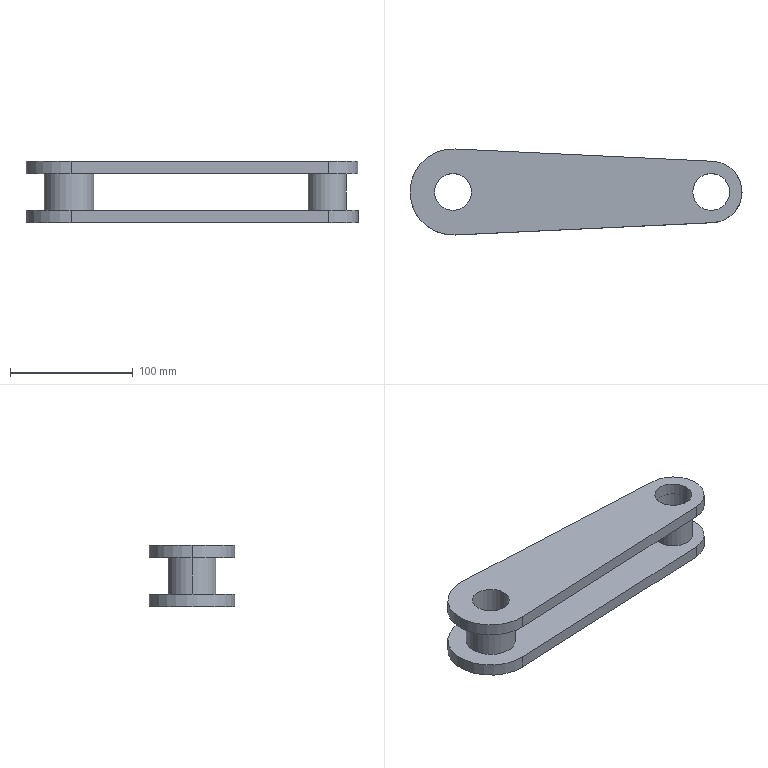Part | SolidWorks | features ICE 4, Extrusion 1 | 2 solids | 28 faces | box 270 x 70 x 50 mm | volume 300062 mm3 | cylinder 18 | plane 10 | commonest cylinder face diameters 30 x8 50 x3 70 x3 31 x2 40 x2
STEP:
#1=CARTESIAN_POINT('',(225.,0.,-30.));
#2=VERTEX_POINT('',#1);
#3=CARTESIAN_POINT('',(195.,0.,-30.));
#4=VERTEX_POINT('',#3);
#5=CARTESIAN_POINT('',(210.,0.,-30.));
#6=DIRECTION('',(0.,0.,-1.));
#7=DIRECTION('',(-1.,0.,0.));
#8=AXIS2_PLACEMENT_3D('',#5,#6,#7);
#9=CIRCLE('',#8,15.);
#10=EDGE_CURVE('',#2,#4,#9,.T.);
#11=ORIENTED_EDGE('',*,*,#10,.T.);
#12=CARTESIAN_POINT('',(195.,0.,10.));
#13=VERTEX_POINT('',#12);
#14=CARTESIAN_POINT('',(195.,0.,-30.));
#15=DIRECTION('',(0.,0.,1.));
#16=VECTOR('',#15,1000.);
#17=LINE('',#14,#16);
#18=EDGE_CURVE('',#4,#13,#17,.T.);
#19=ORIENTED_EDGE('',*,*,#18,.T.);
#20=CARTESIAN_POINT('',(225.,0.,10.));
#21=VERTEX_POINT('',#20);
#22=CARTESIAN_POINT('',(210.,0.,10.));
#23=DIRECTION('',(0.,0.,1.));
#24=DIRECTION('',(1.,0.,0.));
#25=AXIS2_PLACEMENT_3D('',#22,#23,#24);
#26=CIRCLE('',#25,15.);
#27=EDGE_CURVE('',#13,#21,#26,.T.);
#28=ORIENTED_EDGE('',*,*,#27,.T.);
#29=CARTESIAN_POINT('',(225.,0.,-30.));
#30=DIRECTION('',(0.,0.,1.));
#31=VECTOR('',#30,1000.);
#32=LINE('',#29,#31);
#33=EDGE_CURVE('',#2,#21,#32,.T.);
#34=ORIENTED_EDGE('',*,*,#33,.F.);
#35=EDGE_LOOP('',(#11,#19,#28,#34));
#36=FACE_OUTER_BOUND('',#35,.T.);
#37=CARTESIAN_POINT('',(210.,0.,-30.));
#38=DIRECTION('',(0.,0.,1.));
#39=DIRECTION('',(1.,0.,0.));
#40=AXIS2_PLACEMENT_3D('',#37,#38,#39);
#41=CYLINDRICAL_SURFACE('',#40,15.);
#42=ADVANCED_FACE('',(#36),#41,.F.);
#43=CARTESIAN_POINT('',(194.5,0.,-30.));
#44=VERTEX_POINT('',#43);
#45=CARTESIAN_POINT('',(225.5,0.,-30.));
#46=VERTEX_POINT('',#45);
#47=CARTESIAN_POINT('',(210.,0.,-30.));
#48=DIRECTION('',(0.,0.,-1.));
#49=DIRECTION('',(-1.,0.,0.));
#50=AXIS2_PLACEMENT_3D('',#47,#48,#49);
#51=CIRCLE('',#50,15.5);
#52=EDGE_CURVE('',#44,#46,#51,.T.);
#53=ORIENTED_EDGE('',*,*,#52,.F.);
#54=CARTESIAN_POINT('',(194.5,0.,0.));
#55=VERTEX_POINT('',#54);
#56=CARTESIAN_POINT('',(194.5,0.,-30.));
#57=DIRECTION('',(0.,0.,1.));
#58=VECTOR('',#57,1000.);
#59=LINE('',#56,#58);
#60=EDGE_CURVE('',#44,#55,#59,.T.);
#61=ORIENTED_EDGE('',*,*,#60,.T.);
#62=CARTESIAN_POINT('',(225.5,0.,0.));
#63=VERTEX_POINT('',#62);
#64=CARTESIAN_POINT('',(210.,0.,0.));
#65=DIRECTION('',(0.,0.,-1.));
#66=DIRECTION('',(1.,0.,0.));
#67=AXIS2_PLACEMENT_3D('',#64,#65,#66);
#68=CIRCLE('',#67,15.5);
#69=EDGE_CURVE('',#55,#63,#68,.T.);
#70=ORIENTED_EDGE('',*,*,#69,.T.);
#71=CARTESIAN_POINT('',(225.5,0.,-30.));
#72=DIRECTION('',(0.,0.,1.));
#73=VECTOR('',#72,1000.);
#74=LINE('',#71,#73);
#75=EDGE_CURVE('',#46,#63,#74,.T.);
#76=ORIENTED_EDGE('',*,*,#75,.F.);
#77=EDGE_LOOP('',(#53,#61,#70,#76));
#78=FACE_OUTER_BOUND('',#77,.T.);
#79=CARTESIAN_POINT('',(210.,0.,-30.));
#80=DIRECTION('',(0.,0.,1.));
#81=DIRECTION('',(1.,0.,0.));
#82=AXIS2_PLACEMENT_3D('',#79,#80,#81);
#83=CYLINDRICAL_SURFACE('',#82,15.5);
#84=ADVANCED_FACE('',(#78),#83,.T.);
#85=CARTESIAN_POINT('',(15.,0.,-30.));
#86=VERTEX_POINT('',#85);
#87=CARTESIAN_POINT('',(-15.,0.,-30.));
#88=VERTEX_POINT('',#87);
#89=CARTESIAN_POINT('',(0.,0.,-30.));
#90=DIRECTION('',(0.,0.,-1.));
#91=DIRECTION('',(-1.,0.,0.));
#92=AXIS2_PLACEMENT_3D('',#89,#90,#91);
#93=CIRCLE('',#92,15.);
#94=EDGE_CURVE('',#86,#88,#93,.T.);
#95=ORIENTED_EDGE('',*,*,#94,.T.);
#96=CARTESIAN_POINT('',(-15.,0.,10.));
#97=VERTEX_POINT('',#96);
#98=CARTESIAN_POINT('',(-15.,0.,-30.));
#99=DIRECTION('',(0.,0.,1.));
#100=VECTOR('',#99,1000.);
#101=LINE('',#98,#100);
#102=EDGE_CURVE('',#88,#97,#101,.T.);
#103=ORIENTED_EDGE('',*,*,#102,.T.);
#104=CARTESIAN_POINT('',(15.,0.,10.));
#105=VERTEX_POINT('',#104);
#106=CARTESIAN_POINT('',(0.,0.,10.));
#107=DIRECTION('',(0.,0.,1.));
#108=DIRECTION('',(1.,0.,0.));
#109=AXIS2_PLACEMENT_3D('',#106,#107,#108);
#110=CIRCLE('',#109,15.);
#111=EDGE_CURVE('',#97,#105,#110,.T.);
#112=ORIENTED_EDGE('',*,*,#111,.T.);
#113=CARTESIAN_POINT('',(15.,0.,-30.));
#114=DIRECTION('',(0.,0.,1.));
#115=VECTOR('',#114,1000.);
#116=LINE('',#113,#115);
#117=EDGE_CURVE('',#86,#105,#116,.T.);
#118=ORIENTED_EDGE('',*,*,#117,.F.);
#119=EDGE_LOOP('',(#95,#103,#112,#118));
#120=FACE_OUTER_BOUND('',#119,.T.);
#121=CARTESIAN_POINT('',(0.,0.,-30.));
#122=DIRECTION('',(0.,0.,1.));
#123=DIRECTION('',(1.,0.,0.));
#124=AXIS2_PLACEMENT_3D('',#121,#122,#123);
#125=CYLINDRICAL_SURFACE('',#124,15.);
#126=ADVANCED_FACE('',(#120),#125,.F.);
#127=CARTESIAN_POINT('',(-20.,0.,-30.));
#128=VERTEX_POINT('',#127);
#129=CARTESIAN_POINT('',(20.,0.,-30.));
#130=VERTEX_POINT('',#129);
#131=CARTESIAN_POINT('',(0.,0.,-30.));
#132=DIRECTION('',(0.,0.,-1.));
#133=DIRECTION('',(-1.,0.,0.));
#134=AXIS2_PLACEMENT_3D('',#131,#132,#133);
#135=CIRCLE('',#134,20.);
#136=EDGE_CURVE('',#128,#130,#135,.T.);
#137=ORIENTED_EDGE('',*,*,#136,.F.);
#138=CARTESIAN_POINT('',(-20.,0.,0.));
#139=VERTEX_POINT('',#138);
#140=CARTESIAN_POINT('',(-20.,0.,-30.));
#141=DIRECTION('',(0.,0.,1.));
#142=VECTOR('',#141,1000.);
#143=LINE('',#140,#142);
#144=EDGE_CURVE('',#128,#139,#143,.T.);
#145=ORIENTED_EDGE('',*,*,#144,.T.);
#146=CARTESIAN_POINT('',(20.,0.,0.));
#147=VERTEX_POINT('',#146);
#148=CARTESIAN_POINT('',(0.,0.,0.));
#149=DIRECTION('',(0.,0.,-1.));
#150=DIRECTION('',(1.,0.,0.));
#151=AXIS2_PLACEMENT_3D('',#148,#149,#150);
#152=CIRCLE('',#151,20.);
#153=EDGE_CURVE('',#139,#147,#152,.T.);
#154=ORIENTED_EDGE('',*,*,#153,.T.);
#155=CARTESIAN_POINT('',(20.,0.,-30.));
#156=DIRECTION('',(0.,0.,1.));
#157=VECTOR('',#156,1000.);
#158=LINE('',#155,#157);
#159=EDGE_CURVE('',#130,#147,#158,.T.);
#160=ORIENTED_EDGE('',*,*,#159,.F.);
#161=EDGE_LOOP('',(#137,#145,#154,#160));
#162=FACE_OUTER_BOUND('',#161,.T.);
#163=CARTESIAN_POINT('',(0.,0.,-30.));
#164=DIRECTION('',(0.,0.,1.));
#165=DIRECTION('',(1.,0.,0.));
#166=AXIS2_PLACEMENT_3D('',#163,#164,#165);
#167=CYLINDRICAL_SURFACE('',#166,20.);
#168=ADVANCED_FACE('',(#162),#167,.T.);
#169=CARTESIAN_POINT('',(-35.,0.,10.));
#170=VERTEX_POINT('',#169);
#171=CARTESIAN_POINT('',(1.667,-34.96,10.));
#172=VERTEX_POINT('',#171);
#173=CARTESIAN_POINT('',(0.,0.,10.));
#174=DIRECTION('',(0.,0.,1.));
#175=DIRECTION('',(1.,0.,0.));
#176=AXIS2_PLACEMENT_3D('',#173,#174,#175);
#177=CIRCLE('',#176,35.);
#178=EDGE_CURVE('',#170,#172,#177,.T.);
#179=ORIENTED_EDGE('',*,*,#178,.F.);
#180=CARTESIAN_POINT('',(-35.,0.,0.));
#181=VERTEX_POINT('',#180);
#182=CARTESIAN_POINT('',(-35.,0.,10.));
#183=DIRECTION('',(0.,0.,-1.));
#184=VECTOR('',#183,1000.);
#185=LINE('',#182,#184);
#186=EDGE_CURVE('',#170,#181,#185,.T.);
#187=ORIENTED_EDGE('',*,*,#186,.T.);
#188=CARTESIAN_POINT('',(1.667,-34.96,0.));
#189=VERTEX_POINT('',#188);
#190=CARTESIAN_POINT('',(0.,0.,0.));
#191=DIRECTION('',(0.,0.,1.));
#192=DIRECTION('',(1.,0.,0.));
#193=AXIS2_PLACEMENT_3D('',#190,#191,#192);
#194=CIRCLE('',#193,35.);
#195=EDGE_CURVE('',#181,#189,#194,.T.);
#196=ORIENTED_EDGE('',*,*,#195,.T.);
#197=CARTESIAN_POINT('',(1.667,-34.96,10.));
#198=DIRECTION('',(0.,0.,-1.));
#199=VECTOR('',#198,1000.);
#200=LINE('',#197,#199);
#201=EDGE_CURVE('',#172,#189,#200,.T.);
#202=ORIENTED_EDGE('',*,*,#201,.F.);
#203=EDGE_LOOP('',(#179,#187,#196,#202));
#204=FACE_OUTER_BOUND('',#203,.T.);
#205=CARTESIAN_POINT('',(0.,0.,10.));
#206=DIRECTION('',(0.,0.,-1.));
#207=DIRECTION('',(-1.,0.,0.));
#208=AXIS2_PLACEMENT_3D('',#205,#206,#207);
#209=CYLINDRICAL_SURFACE('',#208,35.);
#210=ADVANCED_FACE('',(#204),#209,.T.);
#211=ORIENTED_EDGE('',*,*,#186,.F.);
#212=CARTESIAN_POINT('',(1.667,34.96,10.));
#213=VERTEX_POINT('',#212);
#214=CARTESIAN_POINT('',(0.,0.,10.));
#215=DIRECTION('',(0.,0.,1.));
#216=DIRECTION('',(1.,0.,0.));
#217=AXIS2_PLACEMENT_3D('',#214,#215,#216);
#218=CIRCLE('',#217,35.);
#219=EDGE_CURVE('',#213,#170,#218,.T.);
#220=ORIENTED_EDGE('',*,*,#219,.F.);
#221=CARTESIAN_POINT('',(1.667,34.96,0.));
#222=VERTEX_POINT('',#221);
#223=CARTESIAN_POINT('',(1.667,34.96,10.));
#224=DIRECTION('',(0.,0.,-1.));
#225=VECTOR('',#224,1000.);
#226=LINE('',#223,#225);
#227=EDGE_CURVE('',#213,#222,#226,.T.);
#228=ORIENTED_EDGE('',*,*,#227,.T.);
#229=CARTESIAN_POINT('',(0.,0.,0.));
#230=DIRECTION('',(0.,0.,1.));
#231=DIRECTION('',(1.,0.,0.));
#232=AXIS2_PLACEMENT_3D('',#229,#230,#231);
#233=CIRCLE('',#232,35.);
#234=EDGE_CURVE('',#222,#181,#233,.T.);
#235=ORIENTED_EDGE('',*,*,#234,.T.);
#236=EDGE_LOOP('',(#211,#220,#228,#235));
#237=FACE_OUTER_BOUND('',#236,.T.);
#238=CARTESIAN_POINT('',(0.,0.,10.));
#239=DIRECTION('',(0.,0.,-1.));
#240=DIRECTION('',(-1.,0.,0.));
#241=AXIS2_PLACEMENT_3D('',#238,#239,#240);
#242=CYLINDRICAL_SURFACE('',#241,35.);
#243=ADVANCED_FACE('',(#237),#242,.T.);
#244=CARTESIAN_POINT('',(211.19,-24.972,0.));
#245=VERTEX_POINT('',#244);
#246=CARTESIAN_POINT('',(1.667,-34.96,0.));
#247=DIRECTION('',(0.9989,0.04762,0.));
#248=VECTOR('',#247,1000.);
#249=LINE('',#246,#248);
#250=EDGE_CURVE('',#189,#245,#249,.T.);
#251=ORIENTED_EDGE('',*,*,#250,.T.);
#252=CARTESIAN_POINT('',(211.19,-24.972,10.));
#253=VERTEX_POINT('',#252);
#254=CARTESIAN_POINT('',(211.19,-24.972,10.));
#255=DIRECTION('',(0.,0.,-1.));
#256=VECTOR('',#255,1000.);
#257=LINE('',#254,#256);
#258=EDGE_CURVE('',#253,#245,#257,.T.);
#259=ORIENTED_EDGE('',*,*,#258,.F.);
#260=CARTESIAN_POINT('',(1.667,-34.96,10.));
#261=DIRECTION('',(0.9989,0.04762,0.));
#262=VECTOR('',#261,1000.);
#263=LINE('',#260,#262);
#264=EDGE_CURVE('',#172,#253,#263,.T.);
#265=ORIENTED_EDGE('',*,*,#264,.F.);
#266=ORIENTED_EDGE('',*,*,#201,.T.);
#267=EDGE_LOOP('',(#251,#259,#265,#266));
#268=FACE_OUTER_BOUND('',#267,.T.);
#269=CARTESIAN_POINT('',(1.667,-34.96,10.));
#270=DIRECTION('',(-0.04762,0.9989,0.));
#271=DIRECTION('',(-0.9989,-0.04762,0.));
#272=AXIS2_PLACEMENT_3D('',#269,#270,#271);
#273=PLANE('',#272);
#274=ADVANCED_FACE('',(#268),#273,.F.);
#275=CARTESIAN_POINT('',(211.19,24.972,0.));
#276=VERTEX_POINT('',#275);
#277=CARTESIAN_POINT('',(210.,0.,0.));
#278=DIRECTION('',(0.,0.,1.));
#279=DIRECTION('',(1.,0.,0.));
#280=AXIS2_PLACEMENT_3D('',#277,#278,#279);
#281=CIRCLE('',#280,25.);
#282=EDGE_CURVE('',#245,#276,#281,.T.);
#283=ORIENTED_EDGE('',*,*,#282,.T.);
#284=CARTESIAN_POINT('',(211.19,24.972,10.));
#285=VERTEX_POINT('',#284);
#286=CARTESIAN_POINT('',(211.19,24.972,10.));
#287=DIRECTION('',(0.,0.,-1.));
#288=VECTOR('',#287,1000.);
#289=LINE('',#286,#288);
#290=EDGE_CURVE('',#285,#276,#289,.T.);
#291=ORIENTED_EDGE('',*,*,#290,.F.);
#292=CARTESIAN_POINT('',(210.,0.,10.));
#293=DIRECTION('',(0.,0.,1.));
#294=DIRECTION('',(1.,0.,0.));
#295=AXIS2_PLACEMENT_3D('',#292,#293,#294);
#296=CIRCLE('',#295,25.);
#297=EDGE_CURVE('',#253,#285,#296,.T.);
#298=ORIENTED_EDGE('',*,*,#297,.F.);
#299=ORIENTED_EDGE('',*,*,#258,.T.);
#300=EDGE_LOOP('',(#283,#291,#298,#299));
#301=FACE_OUTER_BOUND('',#300,.T.);
#302=CARTESIAN_POINT('',(210.,0.,10.));
#303=DIRECTION('',(0.,0.,-1.));
#304=DIRECTION('',(-1.,0.,0.));
#305=AXIS2_PLACEMENT_3D('',#302,#303,#304);
#306=CYLINDRICAL_SURFACE('',#305,25.);
#307=ADVANCED_FACE('',(#301),#306,.T.);
#308=CARTESIAN_POINT('',(1.667,34.96,0.));
#309=DIRECTION('',(-0.9989,0.04762,0.));
#310=VECTOR('',#309,1000.);
#311=LINE('',#308,#310);
#312=EDGE_CURVE('',#276,#222,#311,.T.);
#313=ORIENTED_EDGE('',*,*,#312,.T.);
#314=ORIENTED_EDGE('',*,*,#227,.F.);
#315=CARTESIAN_POINT('',(1.667,34.96,10.));
#316=DIRECTION('',(-0.9989,0.04762,0.));
#317=VECTOR('',#316,1000.);
#318=LINE('',#315,#317);
#319=EDGE_CURVE('',#285,#213,#318,.T.);
#320=ORIENTED_EDGE('',*,*,#319,.F.);
#321=ORIENTED_EDGE('',*,*,#290,.T.);
#322=EDGE_LOOP('',(#313,#314,#320,#321));
#323=FACE_OUTER_BOUND('',#322,.T.);
#324=CARTESIAN_POINT('',(1.667,34.96,10.));
#325=DIRECTION('',(-0.04762,-0.9989,0.));
#326=DIRECTION('',(0.9989,-0.04762,0.));
#327=AXIS2_PLACEMENT_3D('',#324,#325,#326);
#328=PLANE('',#327);
#329=ADVANCED_FACE('',(#323),#328,.F.);
#330=CARTESIAN_POINT('',(210.,0.,10.));
#331=DIRECTION('',(0.,0.,1.));
#332=DIRECTION('',(1.,0.,0.));
#333=AXIS2_PLACEMENT_3D('',#330,#331,#332);
#334=CIRCLE('',#333,15.);
#335=EDGE_CURVE('',#21,#13,#334,.T.);
#336=ORIENTED_EDGE('',*,*,#335,.F.);
#337=ORIENTED_EDGE('',*,*,#27,.F.);
#338=EDGE_LOOP('',(#336,#337));
#339=FACE_BOUND('',#338,.T.);
#340=CARTESIAN_POINT('',(0.,0.,10.));
#341=DIRECTION('',(0.,0.,1.));
#342=DIRECTION('',(1.,0.,0.));
#343=AXIS2_PLACEMENT_3D('',#340,#341,#342);
#344=CIRCLE('',#343,15.);
#345=EDGE_CURVE('',#105,#97,#344,.T.);
#346=ORIENTED_EDGE('',*,*,#345,.F.);
#347=ORIENTED_EDGE('',*,*,#111,.F.);
#348=EDGE_LOOP('',(#346,#347));
#349=FACE_BOUND('',#348,.T.);
#350=ORIENTED_EDGE('',*,*,#219,.T.);
#351=ORIENTED_EDGE('',*,*,#178,.T.);
#352=ORIENTED_EDGE('',*,*,#264,.T.);
#353=ORIENTED_EDGE('',*,*,#297,.T.);
#354=ORIENTED_EDGE('',*,*,#319,.T.);
#355=EDGE_LOOP('',(#350,#351,#352,#353,#354));
#356=FACE_OUTER_BOUND('',#355,.T.);
#357=CARTESIAN_POINT('',(0.,0.,10.));
#358=DIRECTION('',(0.,0.,1.));
#359=DIRECTION('',(1.,0.,0.));
#360=AXIS2_PLACEMENT_3D('',#357,#358,#359);
#361=PLANE('',#360);
#362=ADVANCED_FACE('',(#339,#349,#356),#361,.T.);
#363=CARTESIAN_POINT('',(210.,0.,0.));
#364=DIRECTION('',(0.,0.,-1.));
#365=DIRECTION('',(1.,0.,0.));
#366=AXIS2_PLACEMENT_3D('',#363,#364,#365);
#367=CIRCLE('',#366,15.5);
#368=EDGE_CURVE('',#63,#55,#367,.T.);
#369=ORIENTED_EDGE('',*,*,#368,.F.);
#370=ORIENTED_EDGE('',*,*,#69,.F.);
#371=EDGE_LOOP('',(#369,#370));
#372=FACE_BOUND('',#371,.T.);
#373=CARTESIAN_POINT('',(0.,0.,0.));
#374=DIRECTION('',(0.,0.,-1.));
#375=DIRECTION('',(1.,0.,0.));
#376=AXIS2_PLACEMENT_3D('',#373,#374,#375);
#377=CIRCLE('',#376,20.);
#378=EDGE_CURVE('',#147,#139,#377,.T.);
#379=ORIENTED_EDGE('',*,*,#378,.F.);
#380=ORIENTED_EDGE('',*,*,#153,.F.);
#381=EDGE_LOOP('',(#379,#380));
#382=FACE_BOUND('',#381,.T.);
#383=ORIENTED_EDGE('',*,*,#234,.F.);
#384=ORIENTED_EDGE('',*,*,#312,.F.);
#385=ORIENTED_EDGE('',*,*,#282,.F.);
#386=ORIENTED_EDGE('',*,*,#250,.F.);
#387=ORIENTED_EDGE('',*,*,#195,.F.);
#388=EDGE_LOOP('',(#383,#384,#385,#386,#387));
#389=FACE_OUTER_BOUND('',#388,.T.);
#390=CARTESIAN_POINT('',(0.,0.,0.));
#391=DIRECTION('',(0.,0.,1.));
#392=DIRECTION('',(1.,0.,0.));
#393=AXIS2_PLACEMENT_3D('',#390,#391,#392);
#394=PLANE('',#393);
#395=ADVANCED_FACE('',(#372,#382,#389),#394,.F.);
#396=CARTESIAN_POINT('',(0.,0.,-30.));
#397=DIRECTION('',(0.,0.,-1.));
#398=DIRECTION('',(-1.,0.,0.));
#399=AXIS2_PLACEMENT_3D('',#396,#397,#398);
#400=CIRCLE('',#399,20.);
#401=EDGE_CURVE('',#130,#128,#400,.T.);
#402=ORIENTED_EDGE('',*,*,#401,.T.);
#403=ORIENTED_EDGE('',*,*,#136,.T.);
#404=EDGE_LOOP('',(#402,#403));
#405=FACE_OUTER_BOUND('',#404,.T.);
#406=ORIENTED_EDGE('',*,*,#94,.F.);
#407=CARTESIAN_POINT('',(0.,0.,-30.));
#408=DIRECTION('',(0.,0.,-1.));
#409=DIRECTION('',(-1.,0.,0.));
#410=AXIS2_PLACEMENT_3D('',#407,#408,#409);
#411=CIRCLE('',#410,15.);
#412=EDGE_CURVE('',#88,#86,#411,.T.);
#413=ORIENTED_EDGE('',*,*,#412,.F.);
#414=EDGE_LOOP('',(#406,#413));
#415=FACE_BOUND('',#414,.T.);
#416=CARTESIAN_POINT('',(0.,0.,-30.));
#417=DIRECTION('',(0.,0.,-1.));
#418=DIRECTION('',(-1.,0.,0.));
#419=AXIS2_PLACEMENT_3D('',#416,#417,#418);
#420=PLANE('',#419);
#421=ADVANCED_FACE('',(#405,#415),#420,.T.);
#422=ORIENTED_EDGE('',*,*,#144,.F.);
#423=ORIENTED_EDGE('',*,*,#401,.F.);
#424=ORIENTED_EDGE('',*,*,#159,.T.);
#425=ORIENTED_EDGE('',*,*,#378,.T.);
#426=EDGE_LOOP('',(#422,#423,#424,#425));
#427=FACE_OUTER_BOUND('',#426,.T.);
#428=CARTESIAN_POINT('',(0.,0.,-30.));
#429=DIRECTION('',(0.,0.,1.));
#430=DIRECTION('',(1.,0.,0.));
#431=AXIS2_PLACEMENT_3D('',#428,#429,#430);
#432=CYLINDRICAL_SURFACE('',#431,20.);
#433=ADVANCED_FACE('',(#427),#432,.T.);
#434=ORIENTED_EDGE('',*,*,#102,.F.);
#435=ORIENTED_EDGE('',*,*,#412,.T.);
#436=ORIENTED_EDGE('',*,*,#117,.T.);
#437=ORIENTED_EDGE('',*,*,#345,.T.);
#438=EDGE_LOOP('',(#434,#435,#436,#437));
#439=FACE_OUTER_BOUND('',#438,.T.);
#440=CARTESIAN_POINT('',(0.,0.,-30.));
#441=DIRECTION('',(0.,0.,1.));
#442=DIRECTION('',(1.,0.,0.));
#443=AXIS2_PLACEMENT_3D('',#440,#441,#442);
#444=CYLINDRICAL_SURFACE('',#443,15.);
#445=ADVANCED_FACE('',(#439),#444,.F.);
#446=CARTESIAN_POINT('',(210.,0.,-30.));
#447=DIRECTION('',(0.,0.,-1.));
#448=DIRECTION('',(-1.,0.,0.));
#449=AXIS2_PLACEMENT_3D('',#446,#447,#448);
#450=CIRCLE('',#449,15.5);
#451=EDGE_CURVE('',#46,#44,#450,.T.);
#452=ORIENTED_EDGE('',*,*,#451,.T.);
#453=ORIENTED_EDGE('',*,*,#52,.T.);
#454=EDGE_LOOP('',(#452,#453));
#455=FACE_OUTER_BOUND('',#454,.T.);
#456=ORIENTED_EDGE('',*,*,#10,.F.);
#457=CARTESIAN_POINT('',(210.,0.,-30.));
#458=DIRECTION('',(0.,0.,-1.));
#459=DIRECTION('',(-1.,0.,0.));
#460=AXIS2_PLACEMENT_3D('',#457,#458,#459);
#461=CIRCLE('',#460,15.);
#462=EDGE_CURVE('',#4,#2,#461,.T.);
#463=ORIENTED_EDGE('',*,*,#462,.F.);
#464=EDGE_LOOP('',(#456,#463));
#465=FACE_BOUND('',#464,.T.);
#466=CARTESIAN_POINT('',(210.,0.,-30.));
#467=DIRECTION('',(0.,0.,-1.));
#468=DIRECTION('',(-1.,0.,0.));
#469=AXIS2_PLACEMENT_3D('',#466,#467,#468);
#470=PLANE('',#469);
#471=ADVANCED_FACE('',(#455,#465),#470,.T.);
#472=ORIENTED_EDGE('',*,*,#60,.F.);
#473=ORIENTED_EDGE('',*,*,#451,.F.);
#474=ORIENTED_EDGE('',*,*,#75,.T.);
#475=ORIENTED_EDGE('',*,*,#368,.T.);
#476=EDGE_LOOP('',(#472,#473,#474,#475));
#477=FACE_OUTER_BOUND('',#476,.T.);
#478=CARTESIAN_POINT('',(210.,0.,-30.));
#479=DIRECTION('',(0.,0.,1.));
#480=DIRECTION('',(1.,0.,0.));
#481=AXIS2_PLACEMENT_3D('',#478,#479,#480);
#482=CYLINDRICAL_SURFACE('',#481,15.5);
#483=ADVANCED_FACE('',(#477),#482,.T.);
#484=ORIENTED_EDGE('',*,*,#18,.F.);
#485=ORIENTED_EDGE('',*,*,#462,.T.);
#486=ORIENTED_EDGE('',*,*,#33,.T.);
#487=ORIENTED_EDGE('',*,*,#335,.T.);
#488=EDGE_LOOP('',(#484,#485,#486,#487));
#489=FACE_OUTER_BOUND('',#488,.T.);
#490=CARTESIAN_POINT('',(210.,0.,-30.));
#491=DIRECTION('',(0.,0.,1.));
#492=DIRECTION('',(1.,0.,0.));
#493=AXIS2_PLACEMENT_3D('',#490,#491,#492);
#494=CYLINDRICAL_SURFACE('',#493,15.);
#495=ADVANCED_FACE('',(#489),#494,.F.);
#496=CLOSED_SHELL('',(#42,#84,#126,#168,#210,#243,#274,#307,#329,#362,#395,#421,#433,#445,#471,#483,#495));
#497=MANIFOLD_SOLID_BREP('',#496);
#498=CARTESIAN_POINT('',(15.,0.,-40.));
#499=VERTEX_POINT('',#498);
#500=CARTESIAN_POINT('',(-15.,0.,-40.));
#501=VERTEX_POINT('',#500);
#502=CARTESIAN_POINT('',(0.,0.,-40.));
#503=DIRECTION('',(0.,0.,-1.));
#504=DIRECTION('',(-1.,0.,0.));
#505=AXIS2_PLACEMENT_3D('',#502,#503,#504);
#506=CIRCLE('',#505,15.);
#507=EDGE_CURVE('',#499,#501,#506,.T.);
#508=ORIENTED_EDGE('',*,*,#507,.T.);
#509=CARTESIAN_POINT('',(-15.,0.,-30.));
#510=VERTEX_POINT('',#509);
#511=CARTESIAN_POINT('',(-15.,0.,-140.));
#512=DIRECTION('',(0.,0.,1.));
#513=VECTOR('',#512,1000.);
#514=LINE('',#511,#513);
#515=EDGE_CURVE('',#501,#510,#514,.T.);
#516=ORIENTED_EDGE('',*,*,#515,.T.);
#517=CARTESIAN_POINT('',(15.,0.,-30.));
#518=VERTEX_POINT('',#517);
#519=CARTESIAN_POINT('',(0.,0.,-30.));
#520=DIRECTION('',(0.,0.,1.));
#521=DIRECTION('',(1.,0.,0.));
#522=AXIS2_PLACEMENT_3D('',#519,#520,#521);
#523=CIRCLE('',#522,15.);
#524=EDGE_CURVE('',#510,#518,#523,.T.);
#525=ORIENTED_EDGE('',*,*,#524,.T.);
#526=CARTESIAN_POINT('',(15.,0.,-140.));
#527=DIRECTION('',(0.,0.,1.));
#528=VECTOR('',#527,1000.);
#529=LINE('',#526,#528);
#530=EDGE_CURVE('',#499,#518,#529,.T.);
#531=ORIENTED_EDGE('',*,*,#530,.F.);
#532=EDGE_LOOP('',(#508,#516,#525,#531));
#533=FACE_OUTER_BOUND('',#532,.T.);
#534=CARTESIAN_POINT('',(0.,0.,-140.));
#535=DIRECTION('',(0.,0.,1.));
#536=DIRECTION('',(1.,0.,0.));
#537=AXIS2_PLACEMENT_3D('',#534,#535,#536);
#538=CYLINDRICAL_SURFACE('',#537,15.);
#539=ADVANCED_FACE('',(#533),#538,.F.);
#540=CARTESIAN_POINT('',(225.,0.,-40.));
#541=VERTEX_POINT('',#540);
#542=CARTESIAN_POINT('',(195.,0.,-40.));
#543=VERTEX_POINT('',#542);
#544=CARTESIAN_POINT('',(210.,0.,-40.));
#545=DIRECTION('',(0.,0.,-1.));
#546=DIRECTION('',(-1.,0.,0.));
#547=AXIS2_PLACEMENT_3D('',#544,#545,#546);
#548=CIRCLE('',#547,15.);
#549=EDGE_CURVE('',#541,#543,#548,.T.);
#550=ORIENTED_EDGE('',*,*,#549,.T.);
#551=CARTESIAN_POINT('',(195.,0.,-30.));
#552=VERTEX_POINT('',#551);
#553=CARTESIAN_POINT('',(195.,0.,-140.));
#554=DIRECTION('',(0.,0.,1.));
#555=VECTOR('',#554,1000.);
#556=LINE('',#553,#555);
#557=EDGE_CURVE('',#543,#552,#556,.T.);
#558=ORIENTED_EDGE('',*,*,#557,.T.);
#559=CARTESIAN_POINT('',(225.,0.,-30.));
#560=VERTEX_POINT('',#559);
#561=CARTESIAN_POINT('',(210.,0.,-30.));
#562=DIRECTION('',(0.,0.,1.));
#563=DIRECTION('',(1.,0.,0.));
#564=AXIS2_PLACEMENT_3D('',#561,#562,#563);
#565=CIRCLE('',#564,15.);
#566=EDGE_CURVE('',#552,#560,#565,.T.);
#567=ORIENTED_EDGE('',*,*,#566,.T.);
#568=CARTESIAN_POINT('',(225.,0.,-140.));
#569=DIRECTION('',(0.,0.,1.));
#570=VECTOR('',#569,1000.);
#571=LINE('',#568,#570);
#572=EDGE_CURVE('',#541,#560,#571,.T.);
#573=ORIENTED_EDGE('',*,*,#572,.F.);
#574=EDGE_LOOP('',(#550,#558,#567,#573));
#575=FACE_OUTER_BOUND('',#574,.T.);
#576=CARTESIAN_POINT('',(210.,0.,-140.));
#577=DIRECTION('',(0.,0.,1.));
#578=DIRECTION('',(1.,0.,0.));
#579=AXIS2_PLACEMENT_3D('',#576,#577,#578);
#580=CYLINDRICAL_SURFACE('',#579,15.);
#581=ADVANCED_FACE('',(#575),#580,.F.);
#582=CARTESIAN_POINT('',(235.,0.,-40.));
#583=VERTEX_POINT('',#582);
#584=CARTESIAN_POINT('',(211.19,-24.972,-40.));
#585=VERTEX_POINT('',#584);
#586=CARTESIAN_POINT('',(210.,0.,-40.));
#587=DIRECTION('',(0.,0.,-1.));
#588=DIRECTION('',(-1.,0.,0.));
#589=AXIS2_PLACEMENT_3D('',#586,#587,#588);
#590=CIRCLE('',#589,25.);
#591=EDGE_CURVE('',#583,#585,#590,.T.);
#592=ORIENTED_EDGE('',*,*,#591,.F.);
#593=CARTESIAN_POINT('',(235.,0.,-30.));
#594=VERTEX_POINT('',#593);
#595=CARTESIAN_POINT('',(235.,0.,-40.));
#596=DIRECTION('',(0.,0.,1.));
#597=VECTOR('',#596,1000.);
#598=LINE('',#595,#597);
#599=EDGE_CURVE('',#583,#594,#598,.T.);
#600=ORIENTED_EDGE('',*,*,#599,.T.);
#601=CARTESIAN_POINT('',(211.19,-24.972,-30.));
#602=VERTEX_POINT('',#601);
#603=CARTESIAN_POINT('',(210.,0.,-30.));
#604=DIRECTION('',(0.,0.,-1.));
#605=DIRECTION('',(-1.,0.,0.));
#606=AXIS2_PLACEMENT_3D('',#603,#604,#605);
#607=CIRCLE('',#606,25.);
#608=EDGE_CURVE('',#594,#602,#607,.T.);
#609=ORIENTED_EDGE('',*,*,#608,.T.);
#610=CARTESIAN_POINT('',(211.19,-24.972,-40.));
#611=DIRECTION('',(0.,0.,1.));
#612=VECTOR('',#611,1000.);
#613=LINE('',#610,#612);
#614=EDGE_CURVE('',#585,#602,#613,.T.);
#615=ORIENTED_EDGE('',*,*,#614,.F.);
#616=EDGE_LOOP('',(#592,#600,#609,#615));
#617=FACE_OUTER_BOUND('',#616,.T.);
#618=CARTESIAN_POINT('',(210.,0.,-40.));
#619=DIRECTION('',(0.,0.,1.));
#620=DIRECTION('',(1.,0.,0.));
#621=AXIS2_PLACEMENT_3D('',#618,#619,#620);
#622=CYLINDRICAL_SURFACE('',#621,25.);
#623=ADVANCED_FACE('',(#617),#622,.T.);
#624=CARTESIAN_POINT('',(1.667,-34.96,-30.));
#625=VERTEX_POINT('',#624);
#626=CARTESIAN_POINT('',(1.667,34.96,-30.));
#627=VERTEX_POINT('',#626);
#628=CARTESIAN_POINT('',(0.,0.,-30.));
#629=DIRECTION('',(0.,0.,-1.));
#630=DIRECTION('',(-1.,0.,0.));
#631=AXIS2_PLACEMENT_3D('',#628,#629,#630);
#632=CIRCLE('',#631,35.);
#633=EDGE_CURVE('',#625,#627,#632,.T.);
#634=ORIENTED_EDGE('',*,*,#633,.T.);
#635=CARTESIAN_POINT('',(1.667,34.96,-40.));
#636=VERTEX_POINT('',#635);
#637=CARTESIAN_POINT('',(1.667,34.96,-40.));
#638=DIRECTION('',(0.,0.,1.));
#639=VECTOR('',#638,1000.);
#640=LINE('',#637,#639);
#641=EDGE_CURVE('',#636,#627,#640,.T.);
#642=ORIENTED_EDGE('',*,*,#641,.F.);
#643=CARTESIAN_POINT('',(1.667,-34.96,-40.));
#644=VERTEX_POINT('',#643);
#645=CARTESIAN_POINT('',(0.,0.,-40.));
#646=DIRECTION('',(0.,0.,-1.));
#647=DIRECTION('',(-1.,0.,0.));
#648=AXIS2_PLACEMENT_3D('',#645,#646,#647);
#649=CIRCLE('',#648,35.);
#650=EDGE_CURVE('',#644,#636,#649,.T.);
#651=ORIENTED_EDGE('',*,*,#650,.F.);
#652=CARTESIAN_POINT('',(1.667,-34.96,-40.));
#653=DIRECTION('',(0.,0.,1.));
#654=VECTOR('',#653,1000.);
#655=LINE('',#652,#654);
#656=EDGE_CURVE('',#644,#625,#655,.T.);
#657=ORIENTED_EDGE('',*,*,#656,.T.);
#658=EDGE_LOOP('',(#634,#642,#651,#657));
#659=FACE_OUTER_BOUND('',#658,.T.);
#660=CARTESIAN_POINT('',(0.,0.,-40.));
#661=DIRECTION('',(0.,0.,1.));
#662=DIRECTION('',(1.,0.,0.));
#663=AXIS2_PLACEMENT_3D('',#660,#661,#662);
#664=CYLINDRICAL_SURFACE('',#663,35.);
#665=ADVANCED_FACE('',(#659),#664,.T.);
#666=CARTESIAN_POINT('',(211.19,24.972,-30.));
#667=VERTEX_POINT('',#666);
#668=CARTESIAN_POINT('',(1.667,34.96,-30.));
#669=DIRECTION('',(0.9989,-0.04762,0.));
#670=VECTOR('',#669,1000.);
#671=LINE('',#668,#670);
#672=EDGE_CURVE('',#627,#667,#671,.T.);
#673=ORIENTED_EDGE('',*,*,#672,.T.);
#674=CARTESIAN_POINT('',(211.19,24.972,-40.));
#675=VERTEX_POINT('',#674);
#676=CARTESIAN_POINT('',(211.19,24.972,-40.));
#677=DIRECTION('',(0.,0.,1.));
#678=VECTOR('',#677,1000.);
#679=LINE('',#676,#678);
#680=EDGE_CURVE('',#675,#667,#679,.T.);
#681=ORIENTED_EDGE('',*,*,#680,.F.);
#682=CARTESIAN_POINT('',(1.667,34.96,-40.));
#683=DIRECTION('',(0.9989,-0.04762,0.));
#684=VECTOR('',#683,1000.);
#685=LINE('',#682,#684);
#686=EDGE_CURVE('',#636,#675,#685,.T.);
#687=ORIENTED_EDGE('',*,*,#686,.F.);
#688=ORIENTED_EDGE('',*,*,#641,.T.);
#689=EDGE_LOOP('',(#673,#681,#687,#688));
#690=FACE_OUTER_BOUND('',#689,.T.);
#691=CARTESIAN_POINT('',(1.667,34.96,-40.));
#692=DIRECTION('',(-0.04762,-0.9989,0.));
#693=DIRECTION('',(0.9989,-0.04762,0.));
#694=AXIS2_PLACEMENT_3D('',#691,#692,#693);
#695=PLANE('',#694);
#696=ADVANCED_FACE('',(#690),#695,.F.);
#697=ORIENTED_EDGE('',*,*,#599,.F.);
#698=CARTESIAN_POINT('',(210.,0.,-40.));
#699=DIRECTION('',(0.,0.,-1.));
#700=DIRECTION('',(-1.,0.,0.));
#701=AXIS2_PLACEMENT_3D('',#698,#699,#700);
#702=CIRCLE('',#701,25.);
#703=EDGE_CURVE('',#675,#583,#702,.T.);
#704=ORIENTED_EDGE('',*,*,#703,.F.);
#705=ORIENTED_EDGE('',*,*,#680,.T.);
#706=CARTESIAN_POINT('',(210.,0.,-30.));
#707=DIRECTION('',(0.,0.,-1.));
#708=DIRECTION('',(-1.,0.,0.));
#709=AXIS2_PLACEMENT_3D('',#706,#707,#708);
#710=CIRCLE('',#709,25.);
#711=EDGE_CURVE('',#667,#594,#710,.T.);
#712=ORIENTED_EDGE('',*,*,#711,.T.);
#713=EDGE_LOOP('',(#697,#704,#705,#712));
#714=FACE_OUTER_BOUND('',#713,.T.);
#715=CARTESIAN_POINT('',(210.,0.,-40.));
#716=DIRECTION('',(0.,0.,1.));
#717=DIRECTION('',(1.,0.,0.));
#718=AXIS2_PLACEMENT_3D('',#715,#716,#717);
#719=CYLINDRICAL_SURFACE('',#718,25.);
#720=ADVANCED_FACE('',(#714),#719,.T.);
#721=CARTESIAN_POINT('',(211.19,-24.972,-30.));
#722=DIRECTION('',(-0.9989,-0.04762,0.));
#723=VECTOR('',#722,1000.);
#724=LINE('',#721,#723);
#725=EDGE_CURVE('',#602,#625,#724,.T.);
#726=ORIENTED_EDGE('',*,*,#725,.T.);
#727=ORIENTED_EDGE('',*,*,#656,.F.);
#728=CARTESIAN_POINT('',(211.19,-24.972,-40.));
#729=DIRECTION('',(-0.9989,-0.04762,0.));
#730=VECTOR('',#729,1000.);
#731=LINE('',#728,#730);
#732=EDGE_CURVE('',#585,#644,#731,.T.);
#733=ORIENTED_EDGE('',*,*,#732,.F.);
#734=ORIENTED_EDGE('',*,*,#614,.T.);
#735=EDGE_LOOP('',(#726,#727,#733,#734));
#736=FACE_OUTER_BOUND('',#735,.T.);
#737=CARTESIAN_POINT('',(211.19,-24.972,-40.));
#738=DIRECTION('',(-0.04762,0.9989,0.));
#739=DIRECTION('',(-0.9989,-0.04762,0.));
#740=AXIS2_PLACEMENT_3D('',#737,#738,#739);
#741=PLANE('',#740);
#742=ADVANCED_FACE('',(#736),#741,.F.);
#743=ORIENTED_EDGE('',*,*,#507,.F.);
#744=CARTESIAN_POINT('',(0.,0.,-40.));
#745=DIRECTION('',(0.,0.,-1.));
#746=DIRECTION('',(-1.,0.,0.));
#747=AXIS2_PLACEMENT_3D('',#744,#745,#746);
#748=CIRCLE('',#747,15.);
#749=EDGE_CURVE('',#501,#499,#748,.T.);
#750=ORIENTED_EDGE('',*,*,#749,.F.);
#751=EDGE_LOOP('',(#743,#750));
#752=FACE_BOUND('',#751,.T.);
#753=ORIENTED_EDGE('',*,*,#549,.F.);
#754=CARTESIAN_POINT('',(210.,0.,-40.));
#755=DIRECTION('',(0.,0.,-1.));
#756=DIRECTION('',(-1.,0.,0.));
#757=AXIS2_PLACEMENT_3D('',#754,#755,#756);
#758=CIRCLE('',#757,15.);
#759=EDGE_CURVE('',#543,#541,#758,.T.);
#760=ORIENTED_EDGE('',*,*,#759,.F.);
#761=EDGE_LOOP('',(#753,#760));
#762=FACE_BOUND('',#761,.T.);
#763=ORIENTED_EDGE('',*,*,#650,.T.);
#764=ORIENTED_EDGE('',*,*,#686,.T.);
#765=ORIENTED_EDGE('',*,*,#703,.T.);
#766=ORIENTED_EDGE('',*,*,#591,.T.);
#767=ORIENTED_EDGE('',*,*,#732,.T.);
#768=EDGE_LOOP('',(#763,#764,#765,#766,#767));
#769=FACE_OUTER_BOUND('',#768,.T.);
#770=CARTESIAN_POINT('',(0.,0.,-40.));
#771=DIRECTION('',(0.,0.,-1.));
#772=DIRECTION('',(-1.,0.,0.));
#773=AXIS2_PLACEMENT_3D('',#770,#771,#772);
#774=PLANE('',#773);
#775=ADVANCED_FACE('',(#752,#762,#769),#774,.T.);
#776=CARTESIAN_POINT('',(0.,0.,-30.));
#777=DIRECTION('',(0.,0.,1.));
#778=DIRECTION('',(1.,0.,0.));
#779=AXIS2_PLACEMENT_3D('',#776,#777,#778);
#780=CIRCLE('',#779,15.);
#781=EDGE_CURVE('',#518,#510,#780,.T.);
#782=ORIENTED_EDGE('',*,*,#781,.F.);
#783=ORIENTED_EDGE('',*,*,#524,.F.);
#784=EDGE_LOOP('',(#782,#783));
#785=FACE_BOUND('',#784,.T.);
#786=CARTESIAN_POINT('',(210.,0.,-30.));
#787=DIRECTION('',(0.,0.,1.));
#788=DIRECTION('',(1.,0.,0.));
#789=AXIS2_PLACEMENT_3D('',#786,#787,#788);
#790=CIRCLE('',#789,15.);
#791=EDGE_CURVE('',#560,#552,#790,.T.);
#792=ORIENTED_EDGE('',*,*,#791,.F.);
#793=ORIENTED_EDGE('',*,*,#566,.F.);
#794=EDGE_LOOP('',(#792,#793));
#795=FACE_BOUND('',#794,.T.);
#796=ORIENTED_EDGE('',*,*,#633,.F.);
#797=ORIENTED_EDGE('',*,*,#725,.F.);
#798=ORIENTED_EDGE('',*,*,#608,.F.);
#799=ORIENTED_EDGE('',*,*,#711,.F.);
#800=ORIENTED_EDGE('',*,*,#672,.F.);
#801=EDGE_LOOP('',(#796,#797,#798,#799,#800));
#802=FACE_OUTER_BOUND('',#801,.T.);
#803=CARTESIAN_POINT('',(0.,0.,-30.));
#804=DIRECTION('',(0.,0.,-1.));
#805=DIRECTION('',(-1.,0.,0.));
#806=AXIS2_PLACEMENT_3D('',#803,#804,#805);
#807=PLANE('',#806);
#808=ADVANCED_FACE('',(#785,#795,#802),#807,.F.);
#809=ORIENTED_EDGE('',*,*,#557,.F.);
#810=ORIENTED_EDGE('',*,*,#759,.T.);
#811=ORIENTED_EDGE('',*,*,#572,.T.);
#812=ORIENTED_EDGE('',*,*,#791,.T.);
#813=EDGE_LOOP('',(#809,#810,#811,#812));
#814=FACE_OUTER_BOUND('',#813,.T.);
#815=CARTESIAN_POINT('',(210.,0.,-140.));
#816=DIRECTION('',(0.,0.,1.));
#817=DIRECTION('',(1.,0.,0.));
#818=AXIS2_PLACEMENT_3D('',#815,#816,#817);
#819=CYLINDRICAL_SURFACE('',#818,15.);
#820=ADVANCED_FACE('',(#814),#819,.F.);
#821=ORIENTED_EDGE('',*,*,#515,.F.);
#822=ORIENTED_EDGE('',*,*,#749,.T.);
#823=ORIENTED_EDGE('',*,*,#530,.T.);
#824=ORIENTED_EDGE('',*,*,#781,.T.);
#825=EDGE_LOOP('',(#821,#822,#823,#824));
#826=FACE_OUTER_BOUND('',#825,.T.);
#827=CARTESIAN_POINT('',(0.,0.,-140.));
#828=DIRECTION('',(0.,0.,1.));
#829=DIRECTION('',(1.,0.,0.));
#830=AXIS2_PLACEMENT_3D('',#827,#828,#829);
#831=CYLINDRICAL_SURFACE('',#830,15.);
#832=ADVANCED_FACE('',(#826),#831,.F.);
#833=CLOSED_SHELL('',(#539,#581,#623,#665,#696,#720,#742,#775,#808,#820,#832));
#834=MANIFOLD_SOLID_BREP('',#833);
#835=CARTESIAN_POINT('',(0.,0.,0.));
#836=DIRECTION('',(0.,0.,1.));
#837=DIRECTION('',(1.,0.,0.));
#838=AXIS2_PLACEMENT_3D('',#835,#836,#837);
#839=(LENGTH_UNIT()NAMED_UNIT(*)SI_UNIT(.MILLI.,.METRE.));
#840=UNCERTAINTY_MEASURE_WITH_UNIT(LENGTH_MEASURE(0.00001),#839,'','');
#841=(NAMED_UNIT(*)PLANE_ANGLE_UNIT()SI_UNIT($,.RADIAN.));
#842=(NAMED_UNIT(*)SI_UNIT($,.STERADIAN.)SOLID_ANGLE_UNIT());
#843=(GEOMETRIC_REPRESENTATION_CONTEXT(3)GLOBAL_UNCERTAINTY_ASSIGNED_CONTEXT((#840))GLOBAL_UNIT_ASSIGNED_CONTEXT((#839,#841,#842))REPRESENTATION_CONTEXT('',''));
#844=ADVANCED_BREP_SHAPE_REPRESENTATION('',(#497,#834,#838),#843);